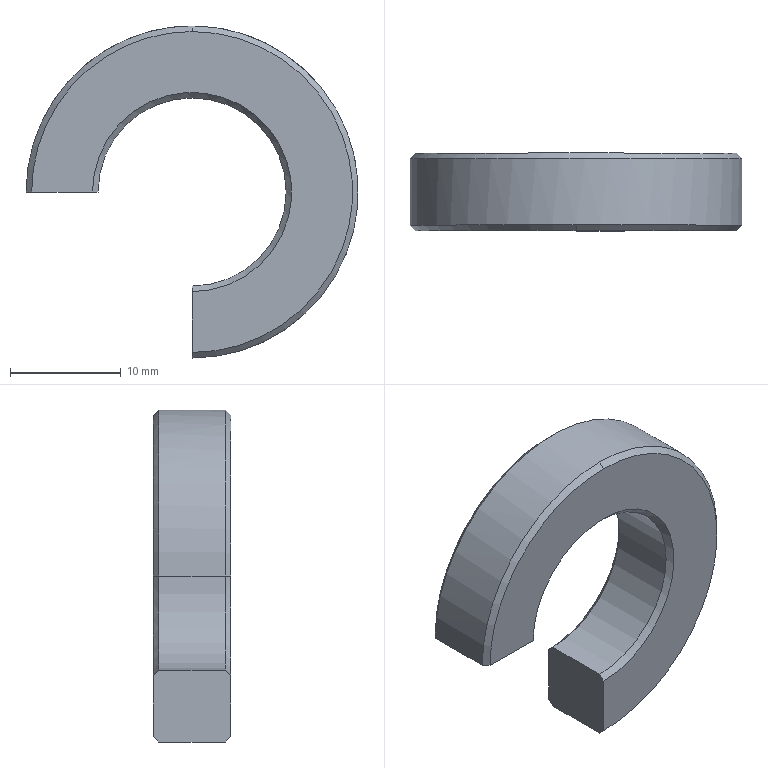Part | STEP file | 6903 ZZ | 1 solid | 12 faces | box 30 x 7 x 30 mm | volume 2492 mm3 | cone 6 | plane 4 | cylinder 2 | commonest cylinder face diameters 17 x1 30 x1
STEP:
#1=CARTESIAN_POINT('',(0.,0.,0.));
#2=DIRECTION('',(0.,0.,1.));
#3=DIRECTION('',(1.,0.,0.));
#4=AXIS2_PLACEMENT_3D('',#1,#2,#3);
#5=CARTESIAN_POINT('',(0.,7.,-9.));
#6=VERTEX_POINT('',#5);
#7=CARTESIAN_POINT('',(0.,6.5,-8.5));
#8=VERTEX_POINT('',#7);
#9=CARTESIAN_POINT('',(0.,-2.,0.));
#10=DIRECTION('',(0.,-0.7071,0.7071));
#11=VECTOR('',#10,1.);
#12=LINE('',#9,#11);
#13=CARTESIAN_POINT('',(0.,6.5,0.));
#14=DIRECTION('',(0.,1.,0.));
#15=DIRECTION('',(0.,0.,1.));
#16=AXIS2_PLACEMENT_3D('',#13,#14,#15);
#17=CONICAL_SURFACE('',#16,8.5,0.7854);
#18=CARTESIAN_POINT('',(3.142,-8.5));
#19=DIRECTION('',(0.,-1.));
#20=VECTOR('',#19,1.);
#21=LINE('',#18,#20);
#22=(GEOMETRIC_REPRESENTATION_CONTEXT(2)PARAMETRIC_REPRESENTATION_CONTEXT()REPRESENTATION_CONTEXT('',''));
#23=DEFINITIONAL_REPRESENTATION('',(#21),#22);
#24=PCURVE('',#17,#23);
#25=CARTESIAN_POINT('',(0.,-56.834,33.935));
#26=DIRECTION('',(-1.,0.,0.));
#27=DIRECTION('',(0.,0.,1.));
#28=AXIS2_PLACEMENT_3D('',#25,#26,#27);
#29=PLANE('',#28);
#30=CARTESIAN_POINT('',(-33.935,54.834));
#31=DIRECTION('',(0.7071,-0.7071));
#32=VECTOR('',#31,1.);
#33=LINE('',#30,#32);
#34=(GEOMETRIC_REPRESENTATION_CONTEXT(2)PARAMETRIC_REPRESENTATION_CONTEXT()REPRESENTATION_CONTEXT('',''));
#35=DEFINITIONAL_REPRESENTATION('',(#33),#34);
#36=PCURVE('',#29,#35);
#37=SURFACE_CURVE('',#12,(#24,#36),.PCURVE_S1.);
#38=EDGE_CURVE('',#6,#8,#37,.T.);
#39=ORIENTED_EDGE('',*,*,#38,.F.);
#40=CARTESIAN_POINT('',(0.,7.,9.));
#41=VERTEX_POINT('',#40);
#42=CARTESIAN_POINT('',(0.,7.,0.));
#43=DIRECTION('',(0.,-1.,0.));
#44=DIRECTION('',(0.,0.,1.));
#45=AXIS2_PLACEMENT_3D('',#42,#43,#44);
#46=CIRCLE('',#45,9.);
#47=CARTESIAN_POINT('',(6.283,0.5));
#48=DIRECTION('',(-1.,0.));
#49=VECTOR('',#48,1.);
#50=LINE('',#47,#49);
#51=(GEOMETRIC_REPRESENTATION_CONTEXT(2)PARAMETRIC_REPRESENTATION_CONTEXT()REPRESENTATION_CONTEXT('',''));
#52=DEFINITIONAL_REPRESENTATION('',(#50),#51);
#53=PCURVE('',#17,#52);
#54=CARTESIAN_POINT('',(0.,7.,0.));
#55=DIRECTION('',(0.,1.,0.));
#56=DIRECTION('',(0.,0.,1.));
#57=AXIS2_PLACEMENT_3D('',#54,#55,#56);
#58=PLANE('',#57);
#59=CARTESIAN_POINT('',(9.,0.));
#60=CARTESIAN_POINT('',(9.,-15.588));
#61=CARTESIAN_POINT('',(-4.5,-7.794));
#62=CARTESIAN_POINT('',(-18.,0.));
#63=CARTESIAN_POINT('',(-4.5,7.794));
#64=CARTESIAN_POINT('',(9.,15.588));
#65=CARTESIAN_POINT('',(9.,0.));
#66=(BOUNDED_CURVE()B_SPLINE_CURVE(2,(#59,#60,#61,#62,#63,#64,#65),.UNSPECIFIED.,.T.,.F.)B_SPLINE_CURVE_WITH_KNOTS((1,2,2,2,2,1),(-2.094,0.,2.094,4.189,6.283,8.378),.UNSPECIFIED.)CURVE()GEOMETRIC_REPRESENTATION_ITEM()RATIONAL_B_SPLINE_CURVE((1.,0.5,1.,0.5,1.,0.5,1.))REPRESENTATION_ITEM(''));
#67=(GEOMETRIC_REPRESENTATION_CONTEXT(2)PARAMETRIC_REPRESENTATION_CONTEXT()REPRESENTATION_CONTEXT('',''));
#68=DEFINITIONAL_REPRESENTATION('',(#66),#67);
#69=PCURVE('',#58,#68);
#70=SURFACE_CURVE('',#46,(#53,#69),.PCURVE_S1.);
#71=EDGE_CURVE('',#6,#41,#70,.T.);
#72=ORIENTED_EDGE('',*,*,#71,.T.);
#73=CARTESIAN_POINT('',(0.,6.5,8.5));
#74=VERTEX_POINT('',#73);
#75=CARTESIAN_POINT('',(0.,6.5,8.5));
#76=DIRECTION('',(0.,0.7071,0.7071));
#77=VECTOR('',#76,1.);
#78=LINE('',#75,#77);
#79=CARTESIAN_POINT('',(0.,0.));
#80=DIRECTION('',(0.,1.));
#81=VECTOR('',#80,1.);
#82=LINE('',#79,#81);
#83=(GEOMETRIC_REPRESENTATION_CONTEXT(2)PARAMETRIC_REPRESENTATION_CONTEXT()REPRESENTATION_CONTEXT('',''));
#84=DEFINITIONAL_REPRESENTATION('',(#82),#83);
#85=PCURVE('',#17,#84);
#86=CARTESIAN_POINT('',(0.,6.5,0.));
#87=DIRECTION('',(0.,1.,0.));
#88=DIRECTION('',(0.,0.,1.));
#89=AXIS2_PLACEMENT_3D('',#86,#87,#88);
#90=CONICAL_SURFACE('',#89,8.5,0.7854);
#91=CARTESIAN_POINT('',(6.283,0.));
#92=DIRECTION('',(0.,1.));
#93=VECTOR('',#92,1.);
#94=LINE('',#91,#93);
#95=(GEOMETRIC_REPRESENTATION_CONTEXT(2)PARAMETRIC_REPRESENTATION_CONTEXT()REPRESENTATION_CONTEXT('',''));
#96=DEFINITIONAL_REPRESENTATION('',(#94),#95);
#97=PCURVE('',#90,#96);
#98=SURFACE_CURVE('',#78,(#85,#97),.PCURVE_S1.);
#99=EDGE_CURVE('',#74,#41,#98,.T.);
#100=ORIENTED_EDGE('',*,*,#99,.F.);
#101=CARTESIAN_POINT('',(0.,6.5,0.));
#102=DIRECTION('',(0.,1.,0.));
#103=DIRECTION('',(0.,0.,1.));
#104=AXIS2_PLACEMENT_3D('',#101,#102,#103);
#105=CIRCLE('',#104,8.5);
#106=CARTESIAN_POINT('',(0.,0.));
#107=DIRECTION('',(1.,0.));
#108=VECTOR('',#107,1.);
#109=LINE('',#106,#108);
#110=(GEOMETRIC_REPRESENTATION_CONTEXT(2)PARAMETRIC_REPRESENTATION_CONTEXT()REPRESENTATION_CONTEXT('',''));
#111=DEFINITIONAL_REPRESENTATION('',(#109),#110);
#112=PCURVE('',#17,#111);
#113=CARTESIAN_POINT('',(0.,7.,0.));
#114=DIRECTION('',(0.,-1.,0.));
#115=DIRECTION('',(0.,0.,-1.));
#116=AXIS2_PLACEMENT_3D('',#113,#114,#115);
#117=CYLINDRICAL_SURFACE('',#116,8.5);
#118=CARTESIAN_POINT('',(3.142,0.5));
#119=DIRECTION('',(-1.,0.));
#120=VECTOR('',#119,1.);
#121=LINE('',#118,#120);
#122=(GEOMETRIC_REPRESENTATION_CONTEXT(2)PARAMETRIC_REPRESENTATION_CONTEXT()REPRESENTATION_CONTEXT('',''));
#123=DEFINITIONAL_REPRESENTATION('',(#121),#122);
#124=PCURVE('',#117,#123);
#125=SURFACE_CURVE('',#105,(#112,#124),.PCURVE_S1.);
#126=EDGE_CURVE('',#74,#8,#125,.T.);
#127=ORIENTED_EDGE('',*,*,#126,.T.);
#128=EDGE_LOOP('',(#39,#72,#100,#127));
#129=FACE_BOUND('',#128,.F.);
#130=ADVANCED_FACE('',(#129),#17,.F.);
#131=CARTESIAN_POINT('',(0.,0.,14.5));
#132=VERTEX_POINT('',#131);
#133=CARTESIAN_POINT('',(-14.5,0.,0.));
#134=VERTEX_POINT('',#133);
#135=CARTESIAN_POINT('',(0.,0.,0.));
#136=DIRECTION('',(0.,-1.,0.));
#137=DIRECTION('',(0.,0.,1.));
#138=AXIS2_PLACEMENT_3D('',#135,#136,#137);
#139=CIRCLE('',#138,14.5);
#140=CARTESIAN_POINT('',(0.,0.5,0.));
#141=DIRECTION('',(0.,1.,0.));
#142=DIRECTION('',(0.,0.,1.));
#143=AXIS2_PLACEMENT_3D('',#140,#141,#142);
#144=CONICAL_SURFACE('',#143,15.,0.7854);
#145=CARTESIAN_POINT('',(6.283,-0.5));
#146=DIRECTION('',(-1.,0.));
#147=VECTOR('',#146,1.);
#148=LINE('',#145,#147);
#149=(GEOMETRIC_REPRESENTATION_CONTEXT(2)PARAMETRIC_REPRESENTATION_CONTEXT()REPRESENTATION_CONTEXT('',''));
#150=DEFINITIONAL_REPRESENTATION('',(#148),#149);
#151=PCURVE('',#144,#150);
#152=CARTESIAN_POINT('',(0.,0.,0.));
#153=DIRECTION('',(0.,1.,0.));
#154=DIRECTION('',(0.,0.,1.));
#155=AXIS2_PLACEMENT_3D('',#152,#153,#154);
#156=PLANE('',#155);
#157=CARTESIAN_POINT('',(14.5,0.));
#158=CARTESIAN_POINT('',(14.5,-25.115));
#159=CARTESIAN_POINT('',(-7.25,-12.557));
#160=CARTESIAN_POINT('',(-29.,0.));
#161=CARTESIAN_POINT('',(-7.25,12.557));
#162=CARTESIAN_POINT('',(14.5,25.115));
#163=CARTESIAN_POINT('',(14.5,0.));
#164=(BOUNDED_CURVE()B_SPLINE_CURVE(2,(#157,#158,#159,#160,#161,#162,#163),.UNSPECIFIED.,.T.,.F.)B_SPLINE_CURVE_WITH_KNOTS((1,2,2,2,2,1),(-2.094,0.,2.094,4.189,6.283,8.378),.UNSPECIFIED.)CURVE()GEOMETRIC_REPRESENTATION_ITEM()RATIONAL_B_SPLINE_CURVE((1.,0.5,1.,0.5,1.,0.5,1.))REPRESENTATION_ITEM(''));
#165=(GEOMETRIC_REPRESENTATION_CONTEXT(2)PARAMETRIC_REPRESENTATION_CONTEXT()REPRESENTATION_CONTEXT('',''));
#166=DEFINITIONAL_REPRESENTATION('',(#164),#165);
#167=PCURVE('',#156,#166);
#168=SURFACE_CURVE('',#139,(#151,#167),.PCURVE_S1.);
#169=EDGE_CURVE('',#132,#134,#168,.T.);
#170=ORIENTED_EDGE('',*,*,#169,.F.);
#171=CARTESIAN_POINT('',(0.,0.5,15.));
#172=VERTEX_POINT('',#171);
#173=CARTESIAN_POINT('',(0.,0.5,15.));
#174=DIRECTION('',(0.,0.7071,0.7071));
#175=VECTOR('',#174,1.);
#176=LINE('',#173,#175);
#177=CARTESIAN_POINT('',(6.283,0.));
#178=DIRECTION('',(0.,1.));
#179=VECTOR('',#178,1.);
#180=LINE('',#177,#179);
#181=(GEOMETRIC_REPRESENTATION_CONTEXT(2)PARAMETRIC_REPRESENTATION_CONTEXT()REPRESENTATION_CONTEXT('',''));
#182=DEFINITIONAL_REPRESENTATION('',(#180),#181);
#183=PCURVE('',#144,#182);
#184=CARTESIAN_POINT('',(0.,0.5,0.));
#185=DIRECTION('',(0.,1.,0.));
#186=DIRECTION('',(0.,0.,1.));
#187=AXIS2_PLACEMENT_3D('',#184,#185,#186);
#188=CONICAL_SURFACE('',#187,15.,0.7854);
#189=CARTESIAN_POINT('',(0.,0.));
#190=DIRECTION('',(0.,1.));
#191=VECTOR('',#190,1.);
#192=LINE('',#189,#191);
#193=(GEOMETRIC_REPRESENTATION_CONTEXT(2)PARAMETRIC_REPRESENTATION_CONTEXT()REPRESENTATION_CONTEXT('',''));
#194=DEFINITIONAL_REPRESENTATION('',(#192),#193);
#195=PCURVE('',#188,#194);
#196=SURFACE_CURVE('',#176,(#183,#195),.PCURVE_S1.);
#197=EDGE_CURVE('',#132,#172,#196,.T.);
#198=ORIENTED_EDGE('',*,*,#197,.T.);
#199=CARTESIAN_POINT('',(-15.,0.5,0.));
#200=VERTEX_POINT('',#199);
#201=CARTESIAN_POINT('',(0.,0.5,0.));
#202=DIRECTION('',(0.,1.,0.));
#203=DIRECTION('',(0.,0.,1.));
#204=AXIS2_PLACEMENT_3D('',#201,#202,#203);
#205=CIRCLE('',#204,15.);
#206=CARTESIAN_POINT('',(0.,0.));
#207=DIRECTION('',(1.,0.));
#208=VECTOR('',#207,1.);
#209=LINE('',#206,#208);
#210=(GEOMETRIC_REPRESENTATION_CONTEXT(2)PARAMETRIC_REPRESENTATION_CONTEXT()REPRESENTATION_CONTEXT('',''));
#211=DEFINITIONAL_REPRESENTATION('',(#209),#210);
#212=PCURVE('',#144,#211);
#213=CARTESIAN_POINT('',(0.,7.,0.));
#214=DIRECTION('',(0.,-1.,0.));
#215=DIRECTION('',(0.,0.,-1.));
#216=AXIS2_PLACEMENT_3D('',#213,#214,#215);
#217=CYLINDRICAL_SURFACE('',#216,15.);
#218=CARTESIAN_POINT('',(9.425,6.5));
#219=DIRECTION('',(-1.,0.));
#220=VECTOR('',#219,1.);
#221=LINE('',#218,#220);
#222=(GEOMETRIC_REPRESENTATION_CONTEXT(2)PARAMETRIC_REPRESENTATION_CONTEXT()REPRESENTATION_CONTEXT('',''));
#223=DEFINITIONAL_REPRESENTATION('',(#221),#222);
#224=PCURVE('',#217,#223);
#225=SURFACE_CURVE('',#205,(#212,#224),.PCURVE_S1.);
#226=EDGE_CURVE('',#200,#172,#225,.T.);
#227=ORIENTED_EDGE('',*,*,#226,.F.);
#228=CARTESIAN_POINT('',(0.,-14.5,0.));
#229=DIRECTION('',(-0.7071,0.7071,0.));
#230=VECTOR('',#229,1.);
#231=LINE('',#228,#230);
#232=CARTESIAN_POINT('',(4.712,-15.));
#233=DIRECTION('',(0.,1.));
#234=VECTOR('',#233,1.);
#235=LINE('',#232,#234);
#236=(GEOMETRIC_REPRESENTATION_CONTEXT(2)PARAMETRIC_REPRESENTATION_CONTEXT()REPRESENTATION_CONTEXT('',''));
#237=DEFINITIONAL_REPRESENTATION('',(#235),#236);
#238=PCURVE('',#144,#237);
#239=CARTESIAN_POINT('',(0.,-45.57,0.));
#240=DIRECTION('',(0.,0.,1.));
#241=DIRECTION('',(1.,0.,0.));
#242=AXIS2_PLACEMENT_3D('',#239,#240,#241);
#243=PLANE('',#242);
#244=CARTESIAN_POINT('',(0.,31.07));
#245=DIRECTION('',(-0.7071,0.7071));
#246=VECTOR('',#245,1.);
#247=LINE('',#244,#246);
#248=(GEOMETRIC_REPRESENTATION_CONTEXT(2)PARAMETRIC_REPRESENTATION_CONTEXT()REPRESENTATION_CONTEXT('',''));
#249=DEFINITIONAL_REPRESENTATION('',(#247),#248);
#250=PCURVE('',#243,#249);
#251=SURFACE_CURVE('',#231,(#238,#250),.PCURVE_S1.);
#252=EDGE_CURVE('',#134,#200,#251,.T.);
#253=ORIENTED_EDGE('',*,*,#252,.F.);
#254=EDGE_LOOP('',(#170,#198,#227,#253));
#255=FACE_BOUND('',#254,.T.);
#256=ADVANCED_FACE('',(#255),#144,.T.);
#257=CARTESIAN_POINT('',(-14.5,7.,0.));
#258=VERTEX_POINT('',#257);
#259=CARTESIAN_POINT('',(-9.,7.,0.));
#260=VERTEX_POINT('',#259);
#261=CARTESIAN_POINT('',(0.,7.,0.));
#262=DIRECTION('',(1.,0.,0.));
#263=VECTOR('',#262,1.);
#264=LINE('',#261,#263);
#265=CARTESIAN_POINT('',(0.,0.));
#266=DIRECTION('',(0.,1.));
#267=VECTOR('',#266,1.);
#268=LINE('',#265,#267);
#269=(GEOMETRIC_REPRESENTATION_CONTEXT(2)PARAMETRIC_REPRESENTATION_CONTEXT()REPRESENTATION_CONTEXT('',''));
#270=DEFINITIONAL_REPRESENTATION('',(#268),#269);
#271=PCURVE('',#58,#270);
#272=CARTESIAN_POINT('',(0.,52.57));
#273=DIRECTION('',(1.,0.));
#274=VECTOR('',#273,1.);
#275=LINE('',#272,#274);
#276=(GEOMETRIC_REPRESENTATION_CONTEXT(2)PARAMETRIC_REPRESENTATION_CONTEXT()REPRESENTATION_CONTEXT('',''));
#277=DEFINITIONAL_REPRESENTATION('',(#275),#276);
#278=PCURVE('',#243,#277);
#279=SURFACE_CURVE('',#264,(#271,#278),.PCURVE_S1.);
#280=EDGE_CURVE('',#258,#260,#279,.T.);
#281=ORIENTED_EDGE('',*,*,#280,.F.);
#282=CARTESIAN_POINT('',(0.,7.,-14.5));
#283=VERTEX_POINT('',#282);
#284=CARTESIAN_POINT('',(0.,7.,0.));
#285=DIRECTION('',(0.,1.,0.));
#286=DIRECTION('',(0.,0.,1.));
#287=AXIS2_PLACEMENT_3D('',#284,#285,#286);
#288=CIRCLE('',#287,14.5);
#289=CARTESIAN_POINT('',(0.,0.));
#290=DIRECTION('',(1.,0.));
#291=AXIS2_PLACEMENT_2D('',#289,#290);
#292=CIRCLE('',#291,14.5);
#293=(GEOMETRIC_REPRESENTATION_CONTEXT(2)PARAMETRIC_REPRESENTATION_CONTEXT()REPRESENTATION_CONTEXT('',''));
#294=DEFINITIONAL_REPRESENTATION('',(#292),#293);
#295=PCURVE('',#58,#294);
#296=CARTESIAN_POINT('',(0.,7.,0.));
#297=DIRECTION('',(0.,-1.,0.));
#298=DIRECTION('',(0.,0.,-1.));
#299=AXIS2_PLACEMENT_3D('',#296,#297,#298);
#300=CONICAL_SURFACE('',#299,14.5,0.7854);
#301=CARTESIAN_POINT('',(9.425,0.));
#302=DIRECTION('',(-1.,0.));
#303=VECTOR('',#302,1.);
#304=LINE('',#301,#303);
#305=(GEOMETRIC_REPRESENTATION_CONTEXT(2)PARAMETRIC_REPRESENTATION_CONTEXT()REPRESENTATION_CONTEXT('',''));
#306=DEFINITIONAL_REPRESENTATION('',(#304),#305);
#307=PCURVE('',#300,#306);
#308=SURFACE_CURVE('',#288,(#295,#307),.PCURVE_S1.);
#309=EDGE_CURVE('',#258,#283,#308,.T.);
#310=ORIENTED_EDGE('',*,*,#309,.T.);
#311=CARTESIAN_POINT('',(0.,7.,0.));
#312=DIRECTION('',(0.,0.,1.));
#313=VECTOR('',#312,1.);
#314=LINE('',#311,#313);
#315=CARTESIAN_POINT('',(0.,0.));
#316=DIRECTION('',(1.,0.));
#317=VECTOR('',#316,1.);
#318=LINE('',#315,#317);
#319=(GEOMETRIC_REPRESENTATION_CONTEXT(2)PARAMETRIC_REPRESENTATION_CONTEXT()REPRESENTATION_CONTEXT('',''));
#320=DEFINITIONAL_REPRESENTATION('',(#318),#319);
#321=PCURVE('',#58,#320);
#322=CARTESIAN_POINT('',(-33.935,63.834));
#323=DIRECTION('',(1.,0.));
#324=VECTOR('',#323,1.);
#325=LINE('',#322,#324);
#326=(GEOMETRIC_REPRESENTATION_CONTEXT(2)PARAMETRIC_REPRESENTATION_CONTEXT()REPRESENTATION_CONTEXT('',''));
#327=DEFINITIONAL_REPRESENTATION('',(#325),#326);
#328=PCURVE('',#29,#327);
#329=SURFACE_CURVE('',#314,(#321,#328),.PCURVE_S1.);
#330=EDGE_CURVE('',#283,#6,#329,.T.);
#331=ORIENTED_EDGE('',*,*,#330,.T.);
#332=ORIENTED_EDGE('',*,*,#71,.T.);
#333=CARTESIAN_POINT('',(0.,7.,0.));
#334=DIRECTION('',(0.,-1.,0.));
#335=DIRECTION('',(0.,0.,1.));
#336=AXIS2_PLACEMENT_3D('',#333,#334,#335);
#337=CIRCLE('',#336,9.);
#338=CARTESIAN_POINT('',(9.,0.));
#339=CARTESIAN_POINT('',(9.,-15.588));
#340=CARTESIAN_POINT('',(-4.5,-7.794));
#341=CARTESIAN_POINT('',(-18.,0.));
#342=CARTESIAN_POINT('',(-4.5,7.794));
#343=CARTESIAN_POINT('',(9.,15.588));
#344=CARTESIAN_POINT('',(9.,0.));
#345=(BOUNDED_CURVE()B_SPLINE_CURVE(2,(#338,#339,#340,#341,#342,#343,#344),.UNSPECIFIED.,.T.,.F.)B_SPLINE_CURVE_WITH_KNOTS((1,2,2,2,2,1),(-2.094,0.,2.094,4.189,6.283,8.378),.UNSPECIFIED.)CURVE()GEOMETRIC_REPRESENTATION_ITEM()RATIONAL_B_SPLINE_CURVE((1.,0.5,1.,0.5,1.,0.5,1.))REPRESENTATION_ITEM(''));
#346=(GEOMETRIC_REPRESENTATION_CONTEXT(2)PARAMETRIC_REPRESENTATION_CONTEXT()REPRESENTATION_CONTEXT('',''));
#347=DEFINITIONAL_REPRESENTATION('',(#345),#346);
#348=PCURVE('',#58,#347);
#349=CARTESIAN_POINT('',(6.283,0.5));
#350=DIRECTION('',(-1.,0.));
#351=VECTOR('',#350,1.);
#352=LINE('',#349,#351);
#353=(GEOMETRIC_REPRESENTATION_CONTEXT(2)PARAMETRIC_REPRESENTATION_CONTEXT()REPRESENTATION_CONTEXT('',''));
#354=DEFINITIONAL_REPRESENTATION('',(#352),#353);
#355=PCURVE('',#90,#354);
#356=SURFACE_CURVE('',#337,(#348,#355),.PCURVE_S1.);
#357=EDGE_CURVE('',#41,#260,#356,.T.);
#358=ORIENTED_EDGE('',*,*,#357,.T.);
#359=EDGE_LOOP('',(#281,#310,#331,#332,#358));
#360=FACE_BOUND('',#359,.T.);
#361=ADVANCED_FACE('',(#360),#58,.T.);
#362=CARTESIAN_POINT('',(0.,0.,-14.5));
#363=VERTEX_POINT('',#362);
#364=CARTESIAN_POINT('',(0.,0.,0.));
#365=DIRECTION('',(0.,-1.,0.));
#366=DIRECTION('',(0.,0.,1.));
#367=AXIS2_PLACEMENT_3D('',#364,#365,#366);
#368=CIRCLE('',#367,14.5);
#369=CARTESIAN_POINT('',(14.5,0.));
#370=CARTESIAN_POINT('',(14.5,-25.115));
#371=CARTESIAN_POINT('',(-7.25,-12.557));
#372=CARTESIAN_POINT('',(-29.,0.));
#373=CARTESIAN_POINT('',(-7.25,12.557));
#374=CARTESIAN_POINT('',(14.5,25.115));
#375=CARTESIAN_POINT('',(14.5,0.));
#376=(BOUNDED_CURVE()B_SPLINE_CURVE(2,(#369,#370,#371,#372,#373,#374,#375),.UNSPECIFIED.,.T.,.F.)B_SPLINE_CURVE_WITH_KNOTS((1,2,2,2,2,1),(-2.094,0.,2.094,4.189,6.283,8.378),.UNSPECIFIED.)CURVE()GEOMETRIC_REPRESENTATION_ITEM()RATIONAL_B_SPLINE_CURVE((1.,0.5,1.,0.5,1.,0.5,1.))REPRESENTATION_ITEM(''));
#377=(GEOMETRIC_REPRESENTATION_CONTEXT(2)PARAMETRIC_REPRESENTATION_CONTEXT()REPRESENTATION_CONTEXT('',''));
#378=DEFINITIONAL_REPRESENTATION('',(#376),#377);
#379=PCURVE('',#156,#378);
#380=CARTESIAN_POINT('',(6.283,-0.5));
#381=DIRECTION('',(-1.,0.));
#382=VECTOR('',#381,1.);
#383=LINE('',#380,#382);
#384=(GEOMETRIC_REPRESENTATION_CONTEXT(2)PARAMETRIC_REPRESENTATION_CONTEXT()REPRESENTATION_CONTEXT('',''));
#385=DEFINITIONAL_REPRESENTATION('',(#383),#384);
#386=PCURVE('',#188,#385);
#387=SURFACE_CURVE('',#368,(#379,#386),.PCURVE_S1.);
#388=EDGE_CURVE('',#363,#132,#387,.T.);
#389=ORIENTED_EDGE('',*,*,#388,.T.);
#390=ORIENTED_EDGE('',*,*,#169,.T.);
#391=CARTESIAN_POINT('',(-9.,0.,0.));
#392=VERTEX_POINT('',#391);
#393=CARTESIAN_POINT('',(0.,0.,0.));
#394=DIRECTION('',(1.,0.,0.));
#395=VECTOR('',#394,1.);
#396=LINE('',#393,#395);
#397=CARTESIAN_POINT('',(0.,0.));
#398=DIRECTION('',(0.,1.));
#399=VECTOR('',#398,1.);
#400=LINE('',#397,#399);
#401=(GEOMETRIC_REPRESENTATION_CONTEXT(2)PARAMETRIC_REPRESENTATION_CONTEXT()REPRESENTATION_CONTEXT('',''));
#402=DEFINITIONAL_REPRESENTATION('',(#400),#401);
#403=PCURVE('',#156,#402);
#404=CARTESIAN_POINT('',(0.,45.57));
#405=DIRECTION('',(1.,0.));
#406=VECTOR('',#405,1.);
#407=LINE('',#404,#406);
#408=(GEOMETRIC_REPRESENTATION_CONTEXT(2)PARAMETRIC_REPRESENTATION_CONTEXT()REPRESENTATION_CONTEXT('',''));
#409=DEFINITIONAL_REPRESENTATION('',(#407),#408);
#410=PCURVE('',#243,#409);
#411=SURFACE_CURVE('',#396,(#403,#410),.PCURVE_S1.);
#412=EDGE_CURVE('',#134,#392,#411,.T.);
#413=ORIENTED_EDGE('',*,*,#412,.T.);
#414=CARTESIAN_POINT('',(0.,0.,-9.));
#415=VERTEX_POINT('',#414);
#416=CARTESIAN_POINT('',(0.,0.,0.));
#417=DIRECTION('',(0.,1.,0.));
#418=DIRECTION('',(0.,0.,1.));
#419=AXIS2_PLACEMENT_3D('',#416,#417,#418);
#420=CIRCLE('',#419,9.);
#421=CARTESIAN_POINT('',(0.,0.));
#422=DIRECTION('',(1.,0.));
#423=AXIS2_PLACEMENT_2D('',#421,#422);
#424=CIRCLE('',#423,9.);
#425=(GEOMETRIC_REPRESENTATION_CONTEXT(2)PARAMETRIC_REPRESENTATION_CONTEXT()REPRESENTATION_CONTEXT('',''));
#426=DEFINITIONAL_REPRESENTATION('',(#424),#425);
#427=PCURVE('',#156,#426);
#428=CARTESIAN_POINT('',(0.,0.,0.));
#429=DIRECTION('',(0.,-1.,0.));
#430=DIRECTION('',(0.,0.,-1.));
#431=AXIS2_PLACEMENT_3D('',#428,#429,#430);
#432=CONICAL_SURFACE('',#431,9.,0.7854);
#433=CARTESIAN_POINT('',(9.425,0.));
#434=DIRECTION('',(-1.,0.));
#435=VECTOR('',#434,1.);
#436=LINE('',#433,#435);
#437=(GEOMETRIC_REPRESENTATION_CONTEXT(2)PARAMETRIC_REPRESENTATION_CONTEXT()REPRESENTATION_CONTEXT('',''));
#438=DEFINITIONAL_REPRESENTATION('',(#436),#437);
#439=PCURVE('',#432,#438);
#440=SURFACE_CURVE('',#420,(#427,#439),.PCURVE_S1.);
#441=EDGE_CURVE('',#392,#415,#440,.T.);
#442=ORIENTED_EDGE('',*,*,#441,.T.);
#443=CARTESIAN_POINT('',(0.,0.,0.));
#444=DIRECTION('',(0.,0.,1.));
#445=VECTOR('',#444,1.);
#446=LINE('',#443,#445);
#447=CARTESIAN_POINT('',(0.,0.));
#448=DIRECTION('',(1.,0.));
#449=VECTOR('',#448,1.);
#450=LINE('',#447,#449);
#451=(GEOMETRIC_REPRESENTATION_CONTEXT(2)PARAMETRIC_REPRESENTATION_CONTEXT()REPRESENTATION_CONTEXT('',''));
#452=DEFINITIONAL_REPRESENTATION('',(#450),#451);
#453=PCURVE('',#156,#452);
#454=CARTESIAN_POINT('',(-33.935,56.834));
#455=DIRECTION('',(1.,0.));
#456=VECTOR('',#455,1.);
#457=LINE('',#454,#456);
#458=(GEOMETRIC_REPRESENTATION_CONTEXT(2)PARAMETRIC_REPRESENTATION_CONTEXT()REPRESENTATION_CONTEXT('',''));
#459=DEFINITIONAL_REPRESENTATION('',(#457),#458);
#460=PCURVE('',#29,#459);
#461=SURFACE_CURVE('',#446,(#453,#460),.PCURVE_S1.);
#462=EDGE_CURVE('',#363,#415,#461,.T.);
#463=ORIENTED_EDGE('',*,*,#462,.F.);
#464=EDGE_LOOP('',(#389,#390,#413,#442,#463));
#465=FACE_BOUND('',#464,.T.);
#466=ADVANCED_FACE('',(#465),#156,.F.);
#467=CARTESIAN_POINT('',(0.,6.5,-15.));
#468=VERTEX_POINT('',#467);
#469=CARTESIAN_POINT('',(-15.,6.5,0.));
#470=VERTEX_POINT('',#469);
#471=CARTESIAN_POINT('',(0.,6.5,0.));
#472=DIRECTION('',(0.,-1.,0.));
#473=DIRECTION('',(0.,0.,1.));
#474=AXIS2_PLACEMENT_3D('',#471,#472,#473);
#475=CIRCLE('',#474,15.);
#476=CARTESIAN_POINT('',(-3.142,0.5));
#477=DIRECTION('',(1.,0.));
#478=VECTOR('',#477,1.);
#479=LINE('',#476,#478);
#480=(GEOMETRIC_REPRESENTATION_CONTEXT(2)PARAMETRIC_REPRESENTATION_CONTEXT()REPRESENTATION_CONTEXT('',''));
#481=DEFINITIONAL_REPRESENTATION('',(#479),#480);
#482=PCURVE('',#217,#481);
#483=CARTESIAN_POINT('',(-3.142,0.5));
#484=DIRECTION('',(1.,0.));
#485=VECTOR('',#484,1.);
#486=LINE('',#483,#485);
#487=(GEOMETRIC_REPRESENTATION_CONTEXT(2)PARAMETRIC_REPRESENTATION_CONTEXT()REPRESENTATION_CONTEXT('',''));
#488=DEFINITIONAL_REPRESENTATION('',(#486),#487);
#489=PCURVE('',#300,#488);
#490=SURFACE_CURVE('',#475,(#482,#489),.PCURVE_S1.);
#491=EDGE_CURVE('',#468,#470,#490,.T.);
#492=ORIENTED_EDGE('',*,*,#491,.T.);
#493=CARTESIAN_POINT('',(-15.,7.,0.));
#494=DIRECTION('',(0.,-1.,0.));
#495=VECTOR('',#494,1.);
#496=LINE('',#493,#495);
#497=CARTESIAN_POINT('',(4.712,0.));
#498=DIRECTION('',(0.,1.));
#499=VECTOR('',#498,1.);
#500=LINE('',#497,#499);
#501=(GEOMETRIC_REPRESENTATION_CONTEXT(2)PARAMETRIC_REPRESENTATION_CONTEXT()REPRESENTATION_CONTEXT('',''));
#502=DEFINITIONAL_REPRESENTATION('',(#500),#501);
#503=PCURVE('',#217,#502);
#504=CARTESIAN_POINT('',(-15.,52.57));
#505=DIRECTION('',(0.,-1.));
#506=VECTOR('',#505,1.);
#507=LINE('',#504,#506);
#508=(GEOMETRIC_REPRESENTATION_CONTEXT(2)PARAMETRIC_REPRESENTATION_CONTEXT()REPRESENTATION_CONTEXT('',''));
#509=DEFINITIONAL_REPRESENTATION('',(#507),#508);
#510=PCURVE('',#243,#509);
#511=SURFACE_CURVE('',#496,(#503,#510),.PCURVE_S1.);
#512=EDGE_CURVE('',#470,#200,#511,.T.);
#513=ORIENTED_EDGE('',*,*,#512,.T.);
#514=ORIENTED_EDGE('',*,*,#226,.T.);
#515=CARTESIAN_POINT('',(0.,0.5,-15.));
#516=VERTEX_POINT('',#515);
#517=CARTESIAN_POINT('',(0.,0.5,0.));
#518=DIRECTION('',(0.,1.,0.));
#519=DIRECTION('',(0.,0.,1.));
#520=AXIS2_PLACEMENT_3D('',#517,#518,#519);
#521=CIRCLE('',#520,15.);
#522=CARTESIAN_POINT('',(3.142,6.5));
#523=DIRECTION('',(-1.,0.));
#524=VECTOR('',#523,1.);
#525=LINE('',#522,#524);
#526=(GEOMETRIC_REPRESENTATION_CONTEXT(2)PARAMETRIC_REPRESENTATION_CONTEXT()REPRESENTATION_CONTEXT('',''));
#527=DEFINITIONAL_REPRESENTATION('',(#525),#526);
#528=PCURVE('',#217,#527);
#529=CARTESIAN_POINT('',(0.,0.));
#530=DIRECTION('',(1.,0.));
#531=VECTOR('',#530,1.);
#532=LINE('',#529,#531);
#533=(GEOMETRIC_REPRESENTATION_CONTEXT(2)PARAMETRIC_REPRESENTATION_CONTEXT()REPRESENTATION_CONTEXT('',''));
#534=DEFINITIONAL_REPRESENTATION('',(#532),#533);
#535=PCURVE('',#188,#534);
#536=SURFACE_CURVE('',#521,(#528,#535),.PCURVE_S1.);
#537=EDGE_CURVE('',#172,#516,#536,.T.);
#538=ORIENTED_EDGE('',*,*,#537,.T.);
#539=CARTESIAN_POINT('',(0.,7.,-15.));
#540=DIRECTION('',(0.,-1.,0.));
#541=VECTOR('',#540,1.);
#542=LINE('',#539,#541);
#543=CARTESIAN_POINT('',(0.,0.));
#544=DIRECTION('',(0.,1.));
#545=VECTOR('',#544,1.);
#546=LINE('',#543,#545);
#547=(GEOMETRIC_REPRESENTATION_CONTEXT(2)PARAMETRIC_REPRESENTATION_CONTEXT()REPRESENTATION_CONTEXT('',''));
#548=DEFINITIONAL_REPRESENTATION('',(#546),#547);
#549=PCURVE('',#217,#548);
#550=CARTESIAN_POINT('',(-48.935,63.834));
#551=DIRECTION('',(0.,-1.));
#552=VECTOR('',#551,1.);
#553=LINE('',#550,#552);
#554=(GEOMETRIC_REPRESENTATION_CONTEXT(2)PARAMETRIC_REPRESENTATION_CONTEXT()REPRESENTATION_CONTEXT('',''));
#555=DEFINITIONAL_REPRESENTATION('',(#553),#554);
#556=PCURVE('',#29,#555);
#557=SURFACE_CURVE('',#542,(#549,#556),.PCURVE_S1.);
#558=EDGE_CURVE('',#468,#516,#557,.T.);
#559=ORIENTED_EDGE('',*,*,#558,.F.);
#560=EDGE_LOOP('',(#492,#513,#514,#538,#559));
#561=FACE_BOUND('',#560,.T.);
#562=ADVANCED_FACE('',(#561),#217,.T.);
#563=CARTESIAN_POINT('',(0.,0.5,-8.5));
#564=VERTEX_POINT('',#563);
#565=CARTESIAN_POINT('',(-8.5,0.5,0.));
#566=VERTEX_POINT('',#565);
#567=CARTESIAN_POINT('',(0.,0.5,0.));
#568=DIRECTION('',(0.,-1.,0.));
#569=DIRECTION('',(0.,0.,1.));
#570=AXIS2_PLACEMENT_3D('',#567,#568,#569);
#571=CIRCLE('',#570,8.5);
#572=CARTESIAN_POINT('',(-3.142,6.5));
#573=DIRECTION('',(1.,0.));
#574=VECTOR('',#573,1.);
#575=LINE('',#572,#574);
#576=(GEOMETRIC_REPRESENTATION_CONTEXT(2)PARAMETRIC_REPRESENTATION_CONTEXT()REPRESENTATION_CONTEXT('',''));
#577=DEFINITIONAL_REPRESENTATION('',(#575),#576);
#578=PCURVE('',#117,#577);
#579=CARTESIAN_POINT('',(-3.142,-0.5));
#580=DIRECTION('',(1.,0.));
#581=VECTOR('',#580,1.);
#582=LINE('',#579,#581);
#583=(GEOMETRIC_REPRESENTATION_CONTEXT(2)PARAMETRIC_REPRESENTATION_CONTEXT()REPRESENTATION_CONTEXT('',''));
#584=DEFINITIONAL_REPRESENTATION('',(#582),#583);
#585=PCURVE('',#432,#584);
#586=SURFACE_CURVE('',#571,(#578,#585),.PCURVE_S1.);
#587=EDGE_CURVE('',#564,#566,#586,.T.);
#588=ORIENTED_EDGE('',*,*,#587,.F.);
#589=CARTESIAN_POINT('',(0.,7.,-8.5));
#590=DIRECTION('',(0.,-1.,0.));
#591=VECTOR('',#590,1.);
#592=LINE('',#589,#591);
#593=CARTESIAN_POINT('',(0.,0.));
#594=DIRECTION('',(0.,1.));
#595=VECTOR('',#594,1.);
#596=LINE('',#593,#595);
#597=(GEOMETRIC_REPRESENTATION_CONTEXT(2)PARAMETRIC_REPRESENTATION_CONTEXT()REPRESENTATION_CONTEXT('',''));
#598=DEFINITIONAL_REPRESENTATION('',(#596),#597);
#599=PCURVE('',#117,#598);
#600=CARTESIAN_POINT('',(-42.435,63.834));
#601=DIRECTION('',(0.,-1.));
#602=VECTOR('',#601,1.);
#603=LINE('',#600,#602);
#604=(GEOMETRIC_REPRESENTATION_CONTEXT(2)PARAMETRIC_REPRESENTATION_CONTEXT()REPRESENTATION_CONTEXT('',''));
#605=DEFINITIONAL_REPRESENTATION('',(#603),#604);
#606=PCURVE('',#29,#605);
#607=SURFACE_CURVE('',#592,(#599,#606),.PCURVE_S1.);
#608=EDGE_CURVE('',#8,#564,#607,.T.);
#609=ORIENTED_EDGE('',*,*,#608,.F.);
#610=ORIENTED_EDGE('',*,*,#126,.F.);
#611=CARTESIAN_POINT('',(-8.5,6.5,0.));
#612=VERTEX_POINT('',#611);
#613=CARTESIAN_POINT('',(0.,6.5,0.));
#614=DIRECTION('',(0.,1.,0.));
#615=DIRECTION('',(0.,0.,1.));
#616=AXIS2_PLACEMENT_3D('',#613,#614,#615);
#617=CIRCLE('',#616,8.5);
#618=CARTESIAN_POINT('',(9.425,0.5));
#619=DIRECTION('',(-1.,0.));
#620=VECTOR('',#619,1.);
#621=LINE('',#618,#620);
#622=(GEOMETRIC_REPRESENTATION_CONTEXT(2)PARAMETRIC_REPRESENTATION_CONTEXT()REPRESENTATION_CONTEXT('',''));
#623=DEFINITIONAL_REPRESENTATION('',(#621),#622);
#624=PCURVE('',#117,#623);
#625=CARTESIAN_POINT('',(0.,0.));
#626=DIRECTION('',(1.,0.));
#627=VECTOR('',#626,1.);
#628=LINE('',#625,#627);
#629=(GEOMETRIC_REPRESENTATION_CONTEXT(2)PARAMETRIC_REPRESENTATION_CONTEXT()REPRESENTATION_CONTEXT('',''));
#630=DEFINITIONAL_REPRESENTATION('',(#628),#629);
#631=PCURVE('',#90,#630);
#632=SURFACE_CURVE('',#617,(#624,#631),.PCURVE_S1.);
#633=EDGE_CURVE('',#612,#74,#632,.T.);
#634=ORIENTED_EDGE('',*,*,#633,.F.);
#635=CARTESIAN_POINT('',(-8.5,7.,0.));
#636=DIRECTION('',(0.,-1.,0.));
#637=VECTOR('',#636,1.);
#638=LINE('',#635,#637);
#639=CARTESIAN_POINT('',(4.712,0.));
#640=DIRECTION('',(0.,1.));
#641=VECTOR('',#640,1.);
#642=LINE('',#639,#641);
#643=(GEOMETRIC_REPRESENTATION_CONTEXT(2)PARAMETRIC_REPRESENTATION_CONTEXT()REPRESENTATION_CONTEXT('',''));
#644=DEFINITIONAL_REPRESENTATION('',(#642),#643);
#645=PCURVE('',#117,#644);
#646=CARTESIAN_POINT('',(-8.5,52.57));
#647=DIRECTION('',(0.,-1.));
#648=VECTOR('',#647,1.);
#649=LINE('',#646,#648);
#650=(GEOMETRIC_REPRESENTATION_CONTEXT(2)PARAMETRIC_REPRESENTATION_CONTEXT()REPRESENTATION_CONTEXT('',''));
#651=DEFINITIONAL_REPRESENTATION('',(#649),#650);
#652=PCURVE('',#243,#651);
#653=SURFACE_CURVE('',#638,(#645,#652),.PCURVE_S1.);
#654=EDGE_CURVE('',#612,#566,#653,.T.);
#655=ORIENTED_EDGE('',*,*,#654,.T.);
#656=EDGE_LOOP('',(#588,#609,#610,#634,#655));
#657=FACE_BOUND('',#656,.F.);
#658=ADVANCED_FACE('',(#657),#117,.F.);
#659=ORIENTED_EDGE('',*,*,#197,.F.);
#660=ORIENTED_EDGE('',*,*,#388,.F.);
#661=CARTESIAN_POINT('',(0.,-14.5,0.));
#662=DIRECTION('',(0.,0.7071,-0.7071));
#663=VECTOR('',#662,1.);
#664=LINE('',#661,#663);
#665=CARTESIAN_POINT('',(3.142,-15.));
#666=DIRECTION('',(0.,1.));
#667=VECTOR('',#666,1.);
#668=LINE('',#665,#667);
#669=(GEOMETRIC_REPRESENTATION_CONTEXT(2)PARAMETRIC_REPRESENTATION_CONTEXT()REPRESENTATION_CONTEXT('',''));
#670=DEFINITIONAL_REPRESENTATION('',(#668),#669);
#671=PCURVE('',#188,#670);
#672=CARTESIAN_POINT('',(-33.935,42.334));
#673=DIRECTION('',(-0.7071,0.7071));
#674=VECTOR('',#673,1.);
#675=LINE('',#672,#674);
#676=(GEOMETRIC_REPRESENTATION_CONTEXT(2)PARAMETRIC_REPRESENTATION_CONTEXT()REPRESENTATION_CONTEXT('',''));
#677=DEFINITIONAL_REPRESENTATION('',(#675),#676);
#678=PCURVE('',#29,#677);
#679=SURFACE_CURVE('',#664,(#671,#678),.PCURVE_S1.);
#680=EDGE_CURVE('',#363,#516,#679,.T.);
#681=ORIENTED_EDGE('',*,*,#680,.T.);
#682=ORIENTED_EDGE('',*,*,#537,.F.);
#683=EDGE_LOOP('',(#659,#660,#681,#682));
#684=FACE_BOUND('',#683,.T.);
#685=ADVANCED_FACE('',(#684),#188,.T.);
#686=ORIENTED_EDGE('',*,*,#441,.T.);
#687=CARTESIAN_POINT('',(0.,9.,0.));
#688=DIRECTION('',(0.,-0.7071,-0.7071));
#689=VECTOR('',#688,1.);
#690=LINE('',#687,#689);
#691=CARTESIAN_POINT('',(0.,-9.));
#692=DIRECTION('',(0.,1.));
#693=VECTOR('',#692,1.);
#694=LINE('',#691,#693);
#695=(GEOMETRIC_REPRESENTATION_CONTEXT(2)PARAMETRIC_REPRESENTATION_CONTEXT()REPRESENTATION_CONTEXT('',''));
#696=DEFINITIONAL_REPRESENTATION('',(#694),#695);
#697=PCURVE('',#432,#696);
#698=CARTESIAN_POINT('',(-33.935,65.834));
#699=DIRECTION('',(-0.7071,-0.7071));
#700=VECTOR('',#699,1.);
#701=LINE('',#698,#700);
#702=(GEOMETRIC_REPRESENTATION_CONTEXT(2)PARAMETRIC_REPRESENTATION_CONTEXT()REPRESENTATION_CONTEXT('',''));
#703=DEFINITIONAL_REPRESENTATION('',(#701),#702);
#704=PCURVE('',#29,#703);
#705=SURFACE_CURVE('',#690,(#697,#704),.PCURVE_S1.);
#706=EDGE_CURVE('',#564,#415,#705,.T.);
#707=ORIENTED_EDGE('',*,*,#706,.F.);
#708=ORIENTED_EDGE('',*,*,#587,.T.);
#709=CARTESIAN_POINT('',(0.,9.,0.));
#710=DIRECTION('',(-0.7071,-0.7071,0.));
#711=VECTOR('',#710,1.);
#712=LINE('',#709,#711);
#713=CARTESIAN_POINT('',(4.712,-9.));
#714=DIRECTION('',(0.,1.));
#715=VECTOR('',#714,1.);
#716=LINE('',#713,#715);
#717=(GEOMETRIC_REPRESENTATION_CONTEXT(2)PARAMETRIC_REPRESENTATION_CONTEXT()REPRESENTATION_CONTEXT('',''));
#718=DEFINITIONAL_REPRESENTATION('',(#716),#717);
#719=PCURVE('',#432,#718);
#720=CARTESIAN_POINT('',(0.,54.57));
#721=DIRECTION('',(-0.7071,-0.7071));
#722=VECTOR('',#721,1.);
#723=LINE('',#720,#722);
#724=(GEOMETRIC_REPRESENTATION_CONTEXT(2)PARAMETRIC_REPRESENTATION_CONTEXT()REPRESENTATION_CONTEXT('',''));
#725=DEFINITIONAL_REPRESENTATION('',(#723),#724);
#726=PCURVE('',#243,#725);
#727=SURFACE_CURVE('',#712,(#719,#726),.PCURVE_S1.);
#728=EDGE_CURVE('',#566,#392,#727,.T.);
#729=ORIENTED_EDGE('',*,*,#728,.T.);
#730=EDGE_LOOP('',(#686,#707,#708,#729));
#731=FACE_BOUND('',#730,.F.);
#732=ADVANCED_FACE('',(#731),#432,.F.);
#733=CARTESIAN_POINT('',(0.,21.5,0.));
#734=DIRECTION('',(0.7071,0.7071,0.));
#735=VECTOR('',#734,1.);
#736=LINE('',#733,#735);
#737=CARTESIAN_POINT('',(4.712,-14.5));
#738=DIRECTION('',(0.,-1.));
#739=VECTOR('',#738,1.);
#740=LINE('',#737,#739);
#741=(GEOMETRIC_REPRESENTATION_CONTEXT(2)PARAMETRIC_REPRESENTATION_CONTEXT()REPRESENTATION_CONTEXT('',''));
#742=DEFINITIONAL_REPRESENTATION('',(#740),#741);
#743=PCURVE('',#300,#742);
#744=CARTESIAN_POINT('',(0.,67.07));
#745=DIRECTION('',(0.7071,0.7071));
#746=VECTOR('',#745,1.);
#747=LINE('',#744,#746);
#748=(GEOMETRIC_REPRESENTATION_CONTEXT(2)PARAMETRIC_REPRESENTATION_CONTEXT()REPRESENTATION_CONTEXT('',''));
#749=DEFINITIONAL_REPRESENTATION('',(#747),#748);
#750=PCURVE('',#243,#749);
#751=SURFACE_CURVE('',#736,(#743,#750),.PCURVE_S1.);
#752=EDGE_CURVE('',#470,#258,#751,.T.);
#753=ORIENTED_EDGE('',*,*,#752,.F.);
#754=ORIENTED_EDGE('',*,*,#491,.F.);
#755=CARTESIAN_POINT('',(0.,21.5,0.));
#756=DIRECTION('',(0.,0.7071,0.7071));
#757=VECTOR('',#756,1.);
#758=LINE('',#755,#757);
#759=CARTESIAN_POINT('',(0.,-14.5));
#760=DIRECTION('',(0.,-1.));
#761=VECTOR('',#760,1.);
#762=LINE('',#759,#761);
#763=(GEOMETRIC_REPRESENTATION_CONTEXT(2)PARAMETRIC_REPRESENTATION_CONTEXT()REPRESENTATION_CONTEXT('',''));
#764=DEFINITIONAL_REPRESENTATION('',(#762),#763);
#765=PCURVE('',#300,#764);
#766=CARTESIAN_POINT('',(-33.935,78.334));
#767=DIRECTION('',(0.7071,0.7071));
#768=VECTOR('',#767,1.);
#769=LINE('',#766,#768);
#770=(GEOMETRIC_REPRESENTATION_CONTEXT(2)PARAMETRIC_REPRESENTATION_CONTEXT()REPRESENTATION_CONTEXT('',''));
#771=DEFINITIONAL_REPRESENTATION('',(#769),#770);
#772=PCURVE('',#29,#771);
#773=SURFACE_CURVE('',#758,(#765,#772),.PCURVE_S1.);
#774=EDGE_CURVE('',#468,#283,#773,.T.);
#775=ORIENTED_EDGE('',*,*,#774,.T.);
#776=ORIENTED_EDGE('',*,*,#309,.F.);
#777=EDGE_LOOP('',(#753,#754,#775,#776));
#778=FACE_BOUND('',#777,.T.);
#779=ADVANCED_FACE('',(#778),#300,.T.);
#780=ORIENTED_EDGE('',*,*,#357,.T.);
#781=CARTESIAN_POINT('',(0.,-2.,0.));
#782=DIRECTION('',(0.7071,-0.7071,0.));
#783=VECTOR('',#782,1.);
#784=LINE('',#781,#783);
#785=CARTESIAN_POINT('',(4.712,-8.5));
#786=DIRECTION('',(0.,-1.));
#787=VECTOR('',#786,1.);
#788=LINE('',#785,#787);
#789=(GEOMETRIC_REPRESENTATION_CONTEXT(2)PARAMETRIC_REPRESENTATION_CONTEXT()REPRESENTATION_CONTEXT('',''));
#790=DEFINITIONAL_REPRESENTATION('',(#788),#789);
#791=PCURVE('',#90,#790);
#792=CARTESIAN_POINT('',(0.,43.57));
#793=DIRECTION('',(0.7071,-0.7071));
#794=VECTOR('',#793,1.);
#795=LINE('',#792,#794);
#796=(GEOMETRIC_REPRESENTATION_CONTEXT(2)PARAMETRIC_REPRESENTATION_CONTEXT()REPRESENTATION_CONTEXT('',''));
#797=DEFINITIONAL_REPRESENTATION('',(#795),#796);
#798=PCURVE('',#243,#797);
#799=SURFACE_CURVE('',#784,(#791,#798),.PCURVE_S1.);
#800=EDGE_CURVE('',#260,#612,#799,.T.);
#801=ORIENTED_EDGE('',*,*,#800,.T.);
#802=ORIENTED_EDGE('',*,*,#633,.T.);
#803=ORIENTED_EDGE('',*,*,#99,.T.);
#804=EDGE_LOOP('',(#780,#801,#802,#803));
#805=FACE_BOUND('',#804,.F.);
#806=ADVANCED_FACE('',(#805),#90,.F.);
#807=ORIENTED_EDGE('',*,*,#462,.T.);
#808=ORIENTED_EDGE('',*,*,#706,.F.);
#809=ORIENTED_EDGE('',*,*,#608,.F.);
#810=ORIENTED_EDGE('',*,*,#38,.F.);
#811=ORIENTED_EDGE('',*,*,#330,.F.);
#812=ORIENTED_EDGE('',*,*,#774,.F.);
#813=ORIENTED_EDGE('',*,*,#558,.T.);
#814=ORIENTED_EDGE('',*,*,#680,.F.);
#815=EDGE_LOOP('',(#807,#808,#809,#810,#811,#812,#813,#814));
#816=FACE_BOUND('',#815,.T.);
#817=ADVANCED_FACE('',(#816),#29,.T.);
#818=ORIENTED_EDGE('',*,*,#252,.T.);
#819=ORIENTED_EDGE('',*,*,#512,.F.);
#820=ORIENTED_EDGE('',*,*,#752,.T.);
#821=ORIENTED_EDGE('',*,*,#280,.T.);
#822=ORIENTED_EDGE('',*,*,#800,.T.);
#823=ORIENTED_EDGE('',*,*,#654,.T.);
#824=ORIENTED_EDGE('',*,*,#728,.T.);
#825=ORIENTED_EDGE('',*,*,#412,.F.);
#826=EDGE_LOOP('',(#818,#819,#820,#821,#822,#823,#824,#825));
#827=FACE_BOUND('',#826,.T.);
#828=ADVANCED_FACE('',(#827),#243,.F.);
#829=CLOSED_SHELL('',(#130,#256,#361,#466,#562,#658,#685,#732,#779,#806,#817,#828));
#830=MANIFOLD_SOLID_BREP('',#829);
#831=(LENGTH_UNIT()NAMED_UNIT(*)SI_UNIT(.MILLI.,.METRE.));
#832=UNCERTAINTY_MEASURE_WITH_UNIT(LENGTH_MEASURE(0.0000001),#831,'','');
#833=(NAMED_UNIT(*)PLANE_ANGLE_UNIT()SI_UNIT($,.RADIAN.));
#834=(NAMED_UNIT(*)SI_UNIT($,.STERADIAN.)SOLID_ANGLE_UNIT());
#835=(GEOMETRIC_REPRESENTATION_CONTEXT(3)GLOBAL_UNCERTAINTY_ASSIGNED_CONTEXT((#832))GLOBAL_UNIT_ASSIGNED_CONTEXT((#831,#833,#834))REPRESENTATION_CONTEXT('',''));
#836=ADVANCED_BREP_SHAPE_REPRESENTATION('',(#4,#830),#835);